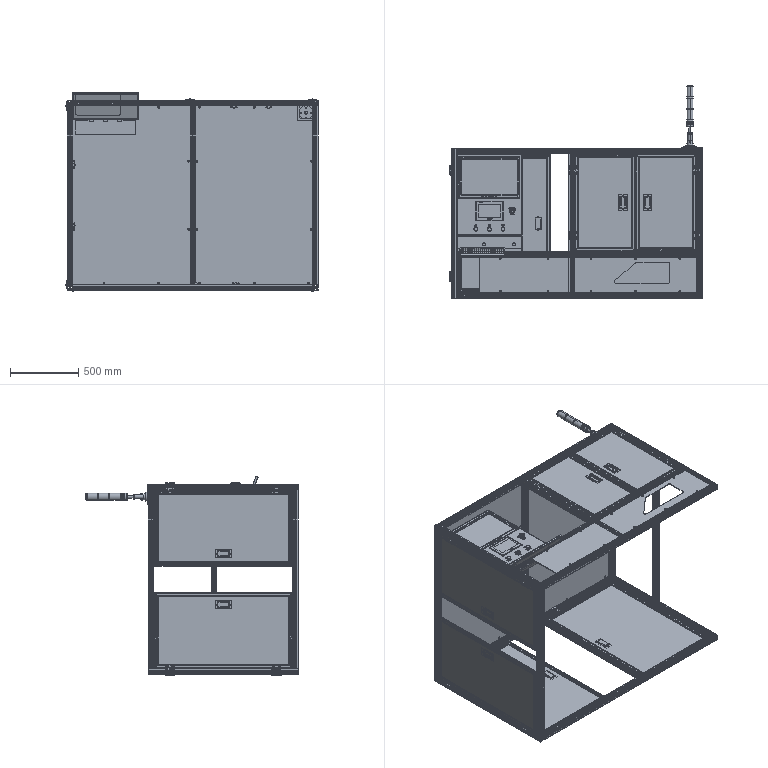Part | SolidWorks | 111 solids | 11175 faces | volume 62540138 mm3 | plane 7071 | cylinder 1821 | spline 1726 | cone 332 | torus 167 | sphere 58 | commonest cylinder face diameters 2 x245 5 x173 8 x170 4 x144 19 x133 10 x106